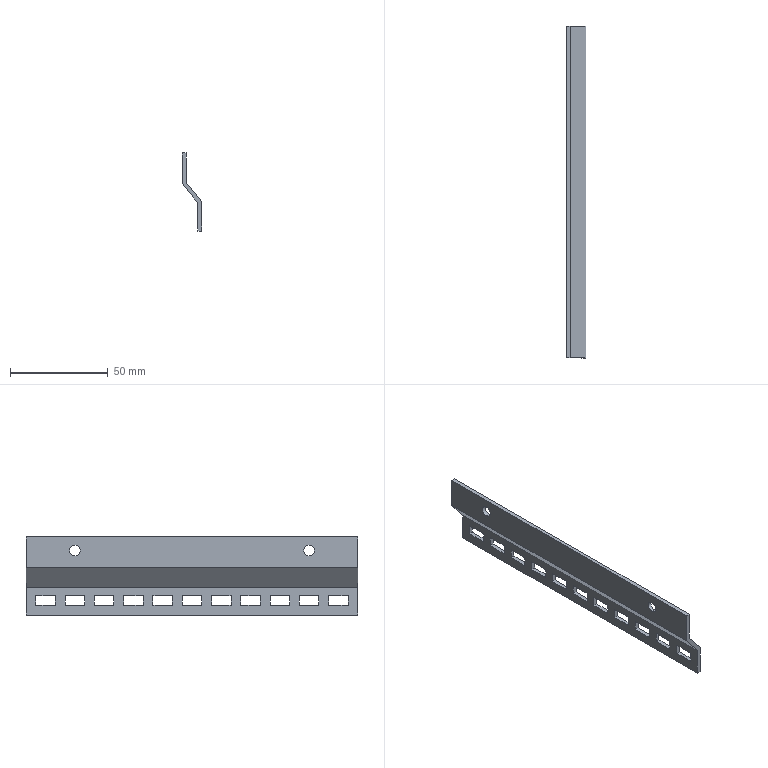Part | SolidWorks | features BaseBody 1 | 1 solid | 58 faces | box 10 x 170 x 40 mm | volume 13359 mm3 | plane 54 | cylinder 4 | commonest cylinder face diameters 5.5 x4